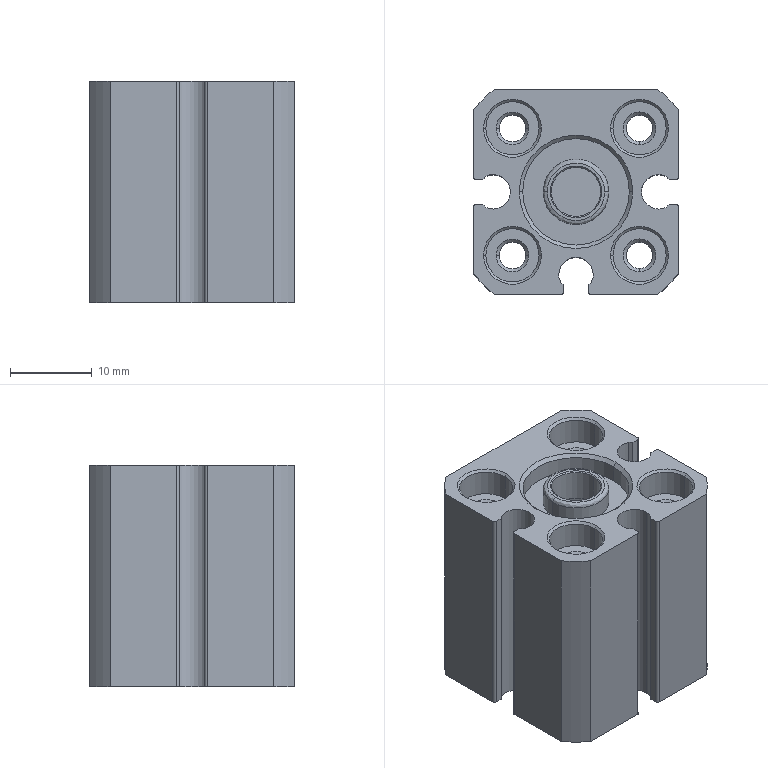Part | STEP file | HI_JSN12X10_body_default | 1 solid | 143 faces | box 25 x 25 x 27 mm | volume 10834 mm3 | cylinder 60 | cone 42 | plane 37 | spline 4 | commonest cylinder face diameters 6.5 x16 3.242 x8 0.6 x6 4.2 x6 1.5 x4 4.134 x4